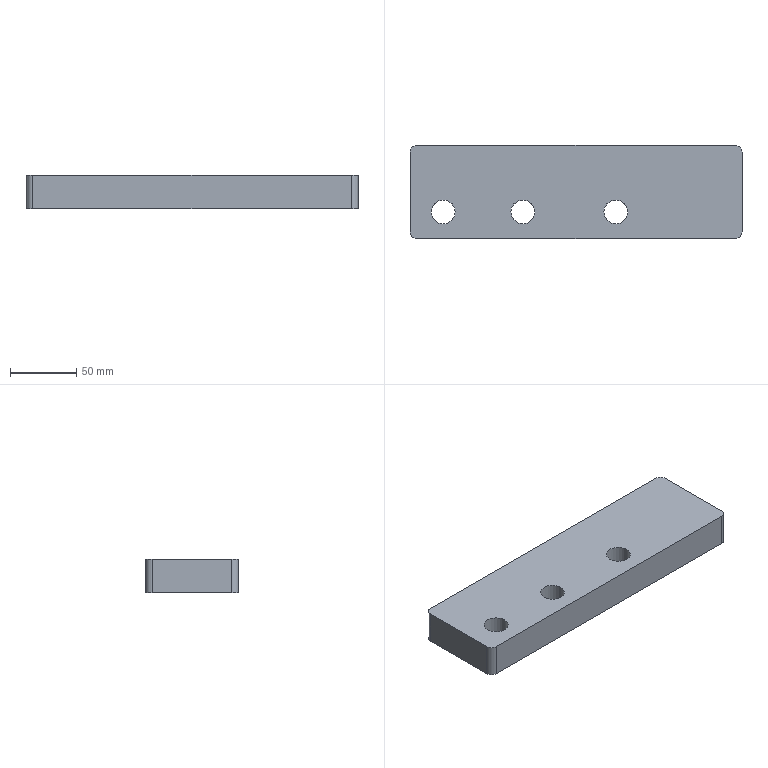Part | NX | features MAIN_BODY 2 | 1 solid | 13 faces | box 250 x 70 x 25 mm | volume 417878 mm3 | cylinder 7 | plane 6 | commonest cylinder face diameters 10 x4 18 x3
STEP:
#1=CARTESIAN_POINT('',(-216.,-257.,-65.));
#2=VERTEX_POINT('',#1);
#3=CARTESIAN_POINT('',(-225.,-257.,-65.));
#4=DIRECTION('',(0.,0.,-1.));
#5=DIRECTION('',(1.,0.,0.));
#6=AXIS2_PLACEMENT_3D('',#3,#4,#5);
#7=CIRCLE('',#6,9.);
#8=EDGE_CURVE('',#2,#2,#7,.F.);
#9=ORIENTED_EDGE('',*,*,#8,.F.);
#10=EDGE_LOOP('',(#9));
#11=FACE_BOUND('',#10,.T.);
#12=CARTESIAN_POINT('',(-294.,-257.,-65.));
#13=VERTEX_POINT('',#12);
#14=CARTESIAN_POINT('',(-285.,-257.,-65.));
#15=DIRECTION('',(0.,0.,-1.));
#16=DIRECTION('',(-1.,0.,0.));
#17=AXIS2_PLACEMENT_3D('',#14,#15,#16);
#18=CIRCLE('',#17,9.);
#19=EDGE_CURVE('',#13,#13,#18,.T.);
#20=ORIENTED_EDGE('',*,*,#19,.T.);
#21=EDGE_LOOP('',(#20));
#22=FACE_BOUND('',#21,.T.);
#23=CARTESIAN_POINT('',(-305.,-207.,-65.));
#24=VERTEX_POINT('',#23);
#25=CARTESIAN_POINT('',(-65.,-207.,-65.));
#26=VERTEX_POINT('',#25);
#27=CARTESIAN_POINT('',(-250.,-207.,-65.));
#28=DIRECTION('',(1.,0.,0.));
#29=VECTOR('',#28,1000.);
#30=LINE('',#27,#29);
#31=EDGE_CURVE('',#24,#26,#30,.T.);
#32=ORIENTED_EDGE('',*,*,#31,.F.);
#33=CARTESIAN_POINT('',(-310.,-212.,-65.));
#34=VERTEX_POINT('',#33);
#35=CARTESIAN_POINT('',(-305.,-212.,-65.));
#36=DIRECTION('',(0.,0.,-1.));
#37=DIRECTION('',(-1.,0.,0.));
#38=AXIS2_PLACEMENT_3D('',#35,#36,#37);
#39=CIRCLE('',#38,5.);
#40=EDGE_CURVE('',#24,#34,#39,.F.);
#41=ORIENTED_EDGE('',*,*,#40,.T.);
#42=CARTESIAN_POINT('',(-310.,-272.,-65.));
#43=VERTEX_POINT('',#42);
#44=CARTESIAN_POINT('',(-310.,-277.,-65.));
#45=DIRECTION('',(0.,1.,0.));
#46=VECTOR('',#45,1000.);
#47=LINE('',#44,#46);
#48=EDGE_CURVE('',#43,#34,#47,.T.);
#49=ORIENTED_EDGE('',*,*,#48,.F.);
#50=CARTESIAN_POINT('',(-305.,-277.,-65.));
#51=VERTEX_POINT('',#50);
#52=CARTESIAN_POINT('',(-305.,-272.,-65.));
#53=DIRECTION('',(0.,0.,-1.));
#54=DIRECTION('',(-1.,0.,0.));
#55=AXIS2_PLACEMENT_3D('',#52,#53,#54);
#56=CIRCLE('',#55,5.);
#57=EDGE_CURVE('',#43,#51,#56,.F.);
#58=ORIENTED_EDGE('',*,*,#57,.T.);
#59=CARTESIAN_POINT('',(-65.,-277.,-65.));
#60=VERTEX_POINT('',#59);
#61=CARTESIAN_POINT('',(-90.,-277.,-65.));
#62=DIRECTION('',(-1.,0.,0.));
#63=VECTOR('',#62,1000.);
#64=LINE('',#61,#63);
#65=EDGE_CURVE('',#60,#51,#64,.T.);
#66=ORIENTED_EDGE('',*,*,#65,.F.);
#67=CARTESIAN_POINT('',(-60.,-272.,-65.));
#68=VERTEX_POINT('',#67);
#69=CARTESIAN_POINT('',(-65.,-272.,-65.));
#70=DIRECTION('',(0.,0.,-1.));
#71=DIRECTION('',(-1.,0.,0.));
#72=AXIS2_PLACEMENT_3D('',#69,#70,#71);
#73=CIRCLE('',#72,5.);
#74=EDGE_CURVE('',#60,#68,#73,.F.);
#75=ORIENTED_EDGE('',*,*,#74,.T.);
#76=CARTESIAN_POINT('',(-60.,-212.,-65.));
#77=VERTEX_POINT('',#76);
#78=CARTESIAN_POINT('',(-60.,-207.,-65.));
#79=DIRECTION('',(0.,-1.,0.));
#80=VECTOR('',#79,1000.);
#81=LINE('',#78,#80);
#82=EDGE_CURVE('',#77,#68,#81,.T.);
#83=ORIENTED_EDGE('',*,*,#82,.F.);
#84=CARTESIAN_POINT('',(-65.,-212.,-65.));
#85=DIRECTION('',(0.,0.,-1.));
#86=DIRECTION('',(-1.,0.,0.));
#87=AXIS2_PLACEMENT_3D('',#84,#85,#86);
#88=CIRCLE('',#87,5.);
#89=EDGE_CURVE('',#77,#26,#88,.F.);
#90=ORIENTED_EDGE('',*,*,#89,.T.);
#91=EDGE_LOOP('',(#32,#41,#49,#58,#66,#75,#83,#90));
#92=FACE_BOUND('',#91,.T.);
#93=CARTESIAN_POINT('',(-164.,-257.,-65.));
#94=VERTEX_POINT('',#93);
#95=CARTESIAN_POINT('',(-155.,-257.,-65.));
#96=DIRECTION('',(0.,0.,-1.));
#97=DIRECTION('',(-1.,0.,0.));
#98=AXIS2_PLACEMENT_3D('',#95,#96,#97);
#99=CIRCLE('',#98,9.);
#100=EDGE_CURVE('',#94,#94,#99,.F.);
#101=ORIENTED_EDGE('',*,*,#100,.F.);
#102=EDGE_LOOP('',(#101));
#103=FACE_BOUND('',#102,.T.);
#104=CARTESIAN_POINT('',(-90.,-277.,-65.));
#105=DIRECTION('',(0.,0.,-1.));
#106=DIRECTION('',(-1.,0.,0.));
#107=AXIS2_PLACEMENT_3D('',#104,#105,#106);
#108=PLANE('',#107);
#109=ADVANCED_FACE('',(#11,#22,#92,#103),#108,.F.);
#110=CARTESIAN_POINT('',(-216.,-257.,-90.));
#111=VERTEX_POINT('',#110);
#112=CARTESIAN_POINT('',(-225.,-257.,-90.));
#113=DIRECTION('',(0.,0.,-1.));
#114=DIRECTION('',(1.,0.,0.));
#115=AXIS2_PLACEMENT_3D('',#112,#113,#114);
#116=CIRCLE('',#115,9.);
#117=EDGE_CURVE('',#111,#111,#116,.F.);
#118=ORIENTED_EDGE('',*,*,#117,.T.);
#119=EDGE_LOOP('',(#118));
#120=FACE_BOUND('',#119,.T.);
#121=CARTESIAN_POINT('',(-294.,-257.,-90.));
#122=VERTEX_POINT('',#121);
#123=CARTESIAN_POINT('',(-285.,-257.,-90.));
#124=DIRECTION('',(0.,0.,-1.));
#125=DIRECTION('',(-1.,0.,0.));
#126=AXIS2_PLACEMENT_3D('',#123,#124,#125);
#127=CIRCLE('',#126,9.);
#128=EDGE_CURVE('',#122,#122,#127,.T.);
#129=ORIENTED_EDGE('',*,*,#128,.F.);
#130=EDGE_LOOP('',(#129));
#131=FACE_BOUND('',#130,.T.);
#132=CARTESIAN_POINT('',(-310.,-272.,-90.));
#133=VERTEX_POINT('',#132);
#134=CARTESIAN_POINT('',(-310.,-212.,-90.));
#135=VERTEX_POINT('',#134);
#136=CARTESIAN_POINT('',(-310.,-277.,-90.));
#137=DIRECTION('',(0.,1.,0.));
#138=VECTOR('',#137,1000.);
#139=LINE('',#136,#138);
#140=EDGE_CURVE('',#133,#135,#139,.T.);
#141=ORIENTED_EDGE('',*,*,#140,.T.);
#142=CARTESIAN_POINT('',(-305.,-207.,-90.));
#143=VERTEX_POINT('',#142);
#144=CARTESIAN_POINT('',(-305.,-212.,-90.));
#145=DIRECTION('',(0.,0.,-1.));
#146=DIRECTION('',(-1.,0.,0.));
#147=AXIS2_PLACEMENT_3D('',#144,#145,#146);
#148=CIRCLE('',#147,5.);
#149=EDGE_CURVE('',#135,#143,#148,.T.);
#150=ORIENTED_EDGE('',*,*,#149,.T.);
#151=CARTESIAN_POINT('',(-65.,-207.,-90.));
#152=VERTEX_POINT('',#151);
#153=CARTESIAN_POINT('',(-250.,-207.,-90.));
#154=DIRECTION('',(1.,0.,0.));
#155=VECTOR('',#154,1000.);
#156=LINE('',#153,#155);
#157=EDGE_CURVE('',#143,#152,#156,.T.);
#158=ORIENTED_EDGE('',*,*,#157,.T.);
#159=CARTESIAN_POINT('',(-60.,-212.,-90.));
#160=VERTEX_POINT('',#159);
#161=CARTESIAN_POINT('',(-65.,-212.,-90.));
#162=DIRECTION('',(0.,0.,-1.));
#163=DIRECTION('',(-1.,0.,0.));
#164=AXIS2_PLACEMENT_3D('',#161,#162,#163);
#165=CIRCLE('',#164,5.);
#166=EDGE_CURVE('',#152,#160,#165,.T.);
#167=ORIENTED_EDGE('',*,*,#166,.T.);
#168=CARTESIAN_POINT('',(-60.,-272.,-90.));
#169=VERTEX_POINT('',#168);
#170=CARTESIAN_POINT('',(-60.,-207.,-90.));
#171=DIRECTION('',(0.,-1.,0.));
#172=VECTOR('',#171,1000.);
#173=LINE('',#170,#172);
#174=EDGE_CURVE('',#160,#169,#173,.T.);
#175=ORIENTED_EDGE('',*,*,#174,.T.);
#176=CARTESIAN_POINT('',(-65.,-277.,-90.));
#177=VERTEX_POINT('',#176);
#178=CARTESIAN_POINT('',(-65.,-272.,-90.));
#179=DIRECTION('',(0.,0.,-1.));
#180=DIRECTION('',(-1.,0.,0.));
#181=AXIS2_PLACEMENT_3D('',#178,#179,#180);
#182=CIRCLE('',#181,5.);
#183=EDGE_CURVE('',#169,#177,#182,.T.);
#184=ORIENTED_EDGE('',*,*,#183,.T.);
#185=CARTESIAN_POINT('',(-305.,-277.,-90.));
#186=VERTEX_POINT('',#185);
#187=CARTESIAN_POINT('',(-90.,-277.,-90.));
#188=DIRECTION('',(-1.,0.,0.));
#189=VECTOR('',#188,1000.);
#190=LINE('',#187,#189);
#191=EDGE_CURVE('',#177,#186,#190,.T.);
#192=ORIENTED_EDGE('',*,*,#191,.T.);
#193=CARTESIAN_POINT('',(-305.,-272.,-90.));
#194=DIRECTION('',(0.,0.,-1.));
#195=DIRECTION('',(-1.,0.,0.));
#196=AXIS2_PLACEMENT_3D('',#193,#194,#195);
#197=CIRCLE('',#196,5.);
#198=EDGE_CURVE('',#186,#133,#197,.T.);
#199=ORIENTED_EDGE('',*,*,#198,.T.);
#200=EDGE_LOOP('',(#141,#150,#158,#167,#175,#184,#192,#199));
#201=FACE_BOUND('',#200,.T.);
#202=CARTESIAN_POINT('',(-164.,-257.,-90.));
#203=VERTEX_POINT('',#202);
#204=CARTESIAN_POINT('',(-155.,-257.,-90.));
#205=DIRECTION('',(0.,0.,-1.));
#206=DIRECTION('',(-1.,0.,0.));
#207=AXIS2_PLACEMENT_3D('',#204,#205,#206);
#208=CIRCLE('',#207,9.);
#209=EDGE_CURVE('',#203,#203,#208,.F.);
#210=ORIENTED_EDGE('',*,*,#209,.T.);
#211=EDGE_LOOP('',(#210));
#212=FACE_BOUND('',#211,.T.);
#213=CARTESIAN_POINT('',(-90.,-277.,-90.));
#214=DIRECTION('',(0.,0.,-1.));
#215=DIRECTION('',(-1.,0.,0.));
#216=AXIS2_PLACEMENT_3D('',#213,#214,#215);
#217=PLANE('',#216);
#218=ADVANCED_FACE('',(#120,#131,#201,#212),#217,.T.);
#219=ORIENTED_EDGE('',*,*,#174,.F.);
#220=CARTESIAN_POINT('',(-60.,-212.,-65.));
#221=DIRECTION('',(0.,0.,-1.));
#222=VECTOR('',#221,1000.);
#223=LINE('',#220,#222);
#224=EDGE_CURVE('',#160,#77,#223,.F.);
#225=ORIENTED_EDGE('',*,*,#224,.T.);
#226=ORIENTED_EDGE('',*,*,#82,.T.);
#227=CARTESIAN_POINT('',(-60.,-272.,-65.));
#228=DIRECTION('',(0.,0.,-1.));
#229=VECTOR('',#228,1000.);
#230=LINE('',#227,#229);
#231=EDGE_CURVE('',#68,#169,#230,.T.);
#232=ORIENTED_EDGE('',*,*,#231,.T.);
#233=EDGE_LOOP('',(#219,#225,#226,#232));
#234=FACE_BOUND('',#233,.T.);
#235=CARTESIAN_POINT('',(-60.,-207.,-65.));
#236=DIRECTION('',(1.,0.,0.));
#237=DIRECTION('',(0.,1.,0.));
#238=AXIS2_PLACEMENT_3D('',#235,#236,#237);
#239=PLANE('',#238);
#240=ADVANCED_FACE('',(#234),#239,.T.);
#241=ORIENTED_EDGE('',*,*,#65,.T.);
#242=CARTESIAN_POINT('',(-305.,-277.,-65.));
#243=DIRECTION('',(0.,0.,-1.));
#244=VECTOR('',#243,1000.);
#245=LINE('',#242,#244);
#246=EDGE_CURVE('',#51,#186,#245,.T.);
#247=ORIENTED_EDGE('',*,*,#246,.T.);
#248=ORIENTED_EDGE('',*,*,#191,.F.);
#249=CARTESIAN_POINT('',(-65.,-277.,-65.));
#250=DIRECTION('',(0.,0.,-1.));
#251=VECTOR('',#250,1000.);
#252=LINE('',#249,#251);
#253=EDGE_CURVE('',#177,#60,#252,.F.);
#254=ORIENTED_EDGE('',*,*,#253,.T.);
#255=EDGE_LOOP('',(#241,#247,#248,#254));
#256=FACE_BOUND('',#255,.T.);
#257=CARTESIAN_POINT('',(-90.,-277.,-65.));
#258=DIRECTION('',(0.,-1.,0.));
#259=DIRECTION('',(1.,0.,0.));
#260=AXIS2_PLACEMENT_3D('',#257,#258,#259);
#261=PLANE('',#260);
#262=ADVANCED_FACE('',(#256),#261,.T.);
#263=ORIENTED_EDGE('',*,*,#48,.T.);
#264=CARTESIAN_POINT('',(-310.,-212.,-65.));
#265=DIRECTION('',(0.,0.,-1.));
#266=VECTOR('',#265,1000.);
#267=LINE('',#264,#266);
#268=EDGE_CURVE('',#34,#135,#267,.T.);
#269=ORIENTED_EDGE('',*,*,#268,.T.);
#270=ORIENTED_EDGE('',*,*,#140,.F.);
#271=CARTESIAN_POINT('',(-310.,-272.,-65.));
#272=DIRECTION('',(0.,0.,-1.));
#273=VECTOR('',#272,1000.);
#274=LINE('',#271,#273);
#275=EDGE_CURVE('',#133,#43,#274,.F.);
#276=ORIENTED_EDGE('',*,*,#275,.T.);
#277=EDGE_LOOP('',(#263,#269,#270,#276));
#278=FACE_BOUND('',#277,.T.);
#279=CARTESIAN_POINT('',(-310.,-277.,-65.));
#280=DIRECTION('',(-1.,0.,0.));
#281=DIRECTION('',(0.,0.,1.));
#282=AXIS2_PLACEMENT_3D('',#279,#280,#281);
#283=PLANE('',#282);
#284=ADVANCED_FACE('',(#278),#283,.T.);
#285=ORIENTED_EDGE('',*,*,#157,.F.);
#286=CARTESIAN_POINT('',(-305.,-207.,-65.));
#287=DIRECTION('',(0.,0.,-1.));
#288=VECTOR('',#287,1000.);
#289=LINE('',#286,#288);
#290=EDGE_CURVE('',#143,#24,#289,.F.);
#291=ORIENTED_EDGE('',*,*,#290,.T.);
#292=ORIENTED_EDGE('',*,*,#31,.T.);
#293=CARTESIAN_POINT('',(-65.,-207.,-65.));
#294=DIRECTION('',(0.,0.,-1.));
#295=VECTOR('',#294,1000.);
#296=LINE('',#293,#295);
#297=EDGE_CURVE('',#26,#152,#296,.T.);
#298=ORIENTED_EDGE('',*,*,#297,.T.);
#299=EDGE_LOOP('',(#285,#291,#292,#298));
#300=FACE_BOUND('',#299,.T.);
#301=CARTESIAN_POINT('',(-250.,-207.,-65.));
#302=DIRECTION('',(0.,1.,0.));
#303=DIRECTION('',(0.,0.,1.));
#304=AXIS2_PLACEMENT_3D('',#301,#302,#303);
#305=PLANE('',#304);
#306=ADVANCED_FACE('',(#300),#305,.T.);
#307=ORIENTED_EDGE('',*,*,#128,.T.);
#308=EDGE_LOOP('',(#307));
#309=FACE_BOUND('',#308,.T.);
#310=ORIENTED_EDGE('',*,*,#19,.F.);
#311=EDGE_LOOP('',(#310));
#312=FACE_BOUND('',#311,.T.);
#313=CARTESIAN_POINT('',(-285.,-257.,-65.));
#314=DIRECTION('',(0.,0.,-1.));
#315=DIRECTION('',(-1.,0.,0.));
#316=AXIS2_PLACEMENT_3D('',#313,#314,#315);
#317=CYLINDRICAL_SURFACE('',#316,9.);
#318=ADVANCED_FACE('',(#309,#312),#317,.F.);
#319=ORIENTED_EDGE('',*,*,#40,.F.);
#320=ORIENTED_EDGE('',*,*,#290,.F.);
#321=ORIENTED_EDGE('',*,*,#149,.F.);
#322=ORIENTED_EDGE('',*,*,#268,.F.);
#323=EDGE_LOOP('',(#319,#320,#321,#322));
#324=FACE_BOUND('',#323,.T.);
#325=CARTESIAN_POINT('',(-305.,-212.,-65.));
#326=DIRECTION('',(0.,0.,-1.));
#327=DIRECTION('',(-1.,0.,0.));
#328=AXIS2_PLACEMENT_3D('',#325,#326,#327);
#329=CYLINDRICAL_SURFACE('',#328,5.);
#330=ADVANCED_FACE('',(#324),#329,.T.);
#331=ORIENTED_EDGE('',*,*,#57,.F.);
#332=ORIENTED_EDGE('',*,*,#275,.F.);
#333=ORIENTED_EDGE('',*,*,#198,.F.);
#334=ORIENTED_EDGE('',*,*,#246,.F.);
#335=EDGE_LOOP('',(#331,#332,#333,#334));
#336=FACE_BOUND('',#335,.T.);
#337=CARTESIAN_POINT('',(-305.,-272.,-65.));
#338=DIRECTION('',(0.,0.,-1.));
#339=DIRECTION('',(-1.,0.,0.));
#340=AXIS2_PLACEMENT_3D('',#337,#338,#339);
#341=CYLINDRICAL_SURFACE('',#340,5.);
#342=ADVANCED_FACE('',(#336),#341,.T.);
#343=ORIENTED_EDGE('',*,*,#89,.F.);
#344=ORIENTED_EDGE('',*,*,#224,.F.);
#345=ORIENTED_EDGE('',*,*,#166,.F.);
#346=ORIENTED_EDGE('',*,*,#297,.F.);
#347=EDGE_LOOP('',(#343,#344,#345,#346));
#348=FACE_BOUND('',#347,.T.);
#349=CARTESIAN_POINT('',(-65.,-212.,-65.));
#350=DIRECTION('',(0.,0.,-1.));
#351=DIRECTION('',(-1.,0.,0.));
#352=AXIS2_PLACEMENT_3D('',#349,#350,#351);
#353=CYLINDRICAL_SURFACE('',#352,5.);
#354=ADVANCED_FACE('',(#348),#353,.T.);
#355=ORIENTED_EDGE('',*,*,#74,.F.);
#356=ORIENTED_EDGE('',*,*,#253,.F.);
#357=ORIENTED_EDGE('',*,*,#183,.F.);
#358=ORIENTED_EDGE('',*,*,#231,.F.);
#359=EDGE_LOOP('',(#355,#356,#357,#358));
#360=FACE_BOUND('',#359,.T.);
#361=CARTESIAN_POINT('',(-65.,-272.,-65.));
#362=DIRECTION('',(0.,0.,-1.));
#363=DIRECTION('',(-1.,0.,0.));
#364=AXIS2_PLACEMENT_3D('',#361,#362,#363);
#365=CYLINDRICAL_SURFACE('',#364,5.);
#366=ADVANCED_FACE('',(#360),#365,.T.);
#367=ORIENTED_EDGE('',*,*,#117,.F.);
#368=EDGE_LOOP('',(#367));
#369=FACE_BOUND('',#368,.T.);
#370=ORIENTED_EDGE('',*,*,#8,.T.);
#371=EDGE_LOOP('',(#370));
#372=FACE_BOUND('',#371,.T.);
#373=CARTESIAN_POINT('',(-225.,-257.,130.));
#374=DIRECTION('',(0.,0.,-1.));
#375=DIRECTION('',(1.,0.,0.));
#376=AXIS2_PLACEMENT_3D('',#373,#374,#375);
#377=CYLINDRICAL_SURFACE('',#376,9.);
#378=ADVANCED_FACE('',(#369,#372),#377,.F.);
#379=ORIENTED_EDGE('',*,*,#209,.F.);
#380=EDGE_LOOP('',(#379));
#381=FACE_BOUND('',#380,.T.);
#382=ORIENTED_EDGE('',*,*,#100,.T.);
#383=EDGE_LOOP('',(#382));
#384=FACE_BOUND('',#383,.T.);
#385=CARTESIAN_POINT('',(-155.,-257.,465.));
#386=DIRECTION('',(0.,0.,-1.));
#387=DIRECTION('',(-1.,0.,0.));
#388=AXIS2_PLACEMENT_3D('',#385,#386,#387);
#389=CYLINDRICAL_SURFACE('',#388,9.);
#390=ADVANCED_FACE('',(#381,#384),#389,.F.);
#391=CLOSED_SHELL('',(#109,#218,#240,#262,#284,#306,#318,#330,#342,#354,#366,#378,#390));
#392=MANIFOLD_SOLID_BREP('',#391);
#393=(LENGTH_UNIT()NAMED_UNIT(*)SI_UNIT(.MILLI.,.METRE.));
#394=UNCERTAINTY_MEASURE_WITH_UNIT(LENGTH_MEASURE(0.00001),#393,'','');
#395=(NAMED_UNIT(*)PLANE_ANGLE_UNIT()SI_UNIT($,.RADIAN.));
#396=(NAMED_UNIT(*)SI_UNIT($,.STERADIAN.)SOLID_ANGLE_UNIT());
#397=(GEOMETRIC_REPRESENTATION_CONTEXT(3)GLOBAL_UNCERTAINTY_ASSIGNED_CONTEXT((#394))GLOBAL_UNIT_ASSIGNED_CONTEXT((#393,#395,#396))REPRESENTATION_CONTEXT('',''));
#398=ADVANCED_BREP_SHAPE_REPRESENTATION('',(#392),#397);